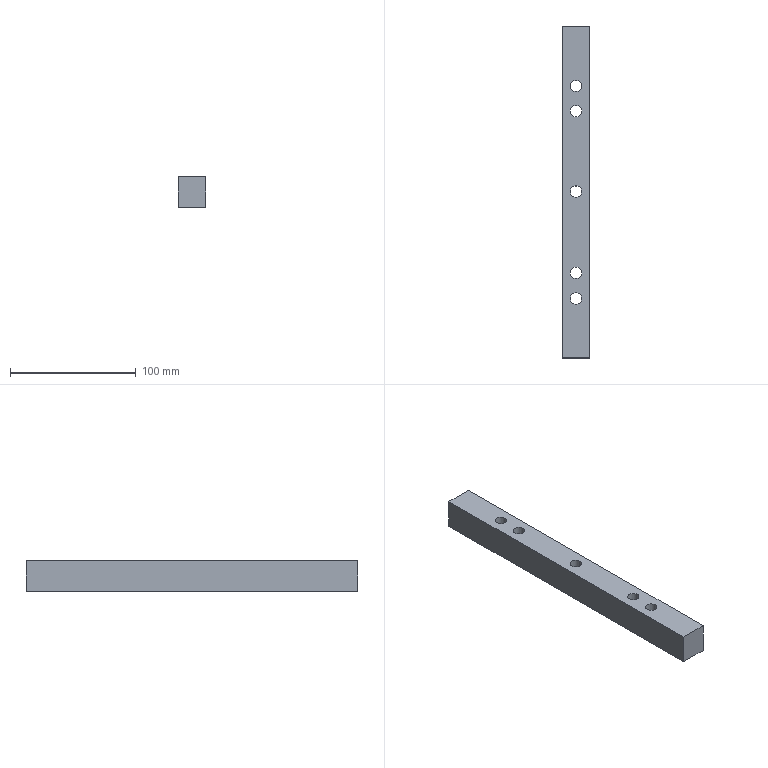Part | NX | features 1605158386 2 | 1 solid | 11 faces | box 22 x 264 x 24 mm | volume 131758 mm3 | plane 6 | cylinder 5 | commonest cylinder face diameters 9 x5
STEP:
#1=CARTESIAN_POINT('',(-281.,-132.15,-46.5));
#2=VERTEX_POINT('',#1);
#3=CARTESIAN_POINT('',(-281.,-132.15,-22.5));
#4=VERTEX_POINT('',#3);
#5=CARTESIAN_POINT('',(-281.,-132.15,-62.5));
#6=DIRECTION('',(0.,0.,1.));
#7=VECTOR('',#6,1000.);
#8=LINE('',#5,#7);
#9=EDGE_CURVE('',#2,#4,#8,.T.);
#10=ORIENTED_EDGE('',*,*,#9,.T.);
#11=CARTESIAN_POINT('',(-303.,-132.15,-22.5));
#12=VERTEX_POINT('',#11);
#13=CARTESIAN_POINT('',(-293.5,-132.15,-22.5));
#14=DIRECTION('',(-1.,0.,0.));
#15=VECTOR('',#14,1000.);
#16=LINE('',#13,#15);
#17=EDGE_CURVE('',#4,#12,#16,.T.);
#18=ORIENTED_EDGE('',*,*,#17,.T.);
#19=CARTESIAN_POINT('',(-303.,-132.15,-46.5));
#20=VERTEX_POINT('',#19);
#21=CARTESIAN_POINT('',(-303.,-132.15,-62.5));
#22=DIRECTION('',(0.,0.,1.));
#23=VECTOR('',#22,1000.);
#24=LINE('',#21,#23);
#25=EDGE_CURVE('',#20,#12,#24,.T.);
#26=ORIENTED_EDGE('',*,*,#25,.F.);
#27=CARTESIAN_POINT('',(-293.5,-132.15,-46.5));
#28=DIRECTION('',(1.,0.,0.));
#29=VECTOR('',#28,1000.);
#30=LINE('',#27,#29);
#31=EDGE_CURVE('',#20,#2,#30,.T.);
#32=ORIENTED_EDGE('',*,*,#31,.T.);
#33=EDGE_LOOP('',(#10,#18,#26,#32));
#34=FACE_BOUND('',#33,.T.);
#35=CARTESIAN_POINT('',(-293.5,-132.15,-62.5));
#36=DIRECTION('',(0.,-1.,0.));
#37=DIRECTION('',(0.,0.,-1.));
#38=AXIS2_PLACEMENT_3D('',#35,#36,#37);
#39=PLANE('',#38);
#40=ADVANCED_FACE('',(#34),#39,.T.);
#41=ORIENTED_EDGE('',*,*,#25,.T.);
#42=CARTESIAN_POINT('',(-303.,131.85,-22.5));
#43=VERTEX_POINT('',#42);
#44=CARTESIAN_POINT('',(-303.,108.85,-22.5));
#45=DIRECTION('',(0.,1.,0.));
#46=VECTOR('',#45,1000.);
#47=LINE('',#44,#46);
#48=EDGE_CURVE('',#12,#43,#47,.T.);
#49=ORIENTED_EDGE('',*,*,#48,.T.);
#50=CARTESIAN_POINT('',(-303.,131.85,-46.5));
#51=VERTEX_POINT('',#50);
#52=CARTESIAN_POINT('',(-303.,131.85,-62.5));
#53=DIRECTION('',(0.,0.,1.));
#54=VECTOR('',#53,1000.);
#55=LINE('',#52,#54);
#56=EDGE_CURVE('',#51,#43,#55,.T.);
#57=ORIENTED_EDGE('',*,*,#56,.F.);
#58=CARTESIAN_POINT('',(-303.,108.85,-46.5));
#59=DIRECTION('',(0.,-1.,0.));
#60=VECTOR('',#59,1000.);
#61=LINE('',#58,#60);
#62=EDGE_CURVE('',#51,#20,#61,.T.);
#63=ORIENTED_EDGE('',*,*,#62,.T.);
#64=EDGE_LOOP('',(#41,#49,#57,#63));
#65=FACE_BOUND('',#64,.T.);
#66=CARTESIAN_POINT('',(-303.,108.85,-62.5));
#67=DIRECTION('',(-1.,0.,0.));
#68=DIRECTION('',(0.,0.,1.));
#69=AXIS2_PLACEMENT_3D('',#66,#67,#68);
#70=PLANE('',#69);
#71=ADVANCED_FACE('',(#65),#70,.T.);
#72=ORIENTED_EDGE('',*,*,#56,.T.);
#73=CARTESIAN_POINT('',(-281.,131.85,-22.5));
#74=VERTEX_POINT('',#73);
#75=CARTESIAN_POINT('',(-293.5,131.85,-22.5));
#76=DIRECTION('',(1.,0.,0.));
#77=VECTOR('',#76,1000.);
#78=LINE('',#75,#77);
#79=EDGE_CURVE('',#43,#74,#78,.T.);
#80=ORIENTED_EDGE('',*,*,#79,.T.);
#81=CARTESIAN_POINT('',(-281.,131.85,-46.5));
#82=VERTEX_POINT('',#81);
#83=CARTESIAN_POINT('',(-281.,131.85,-62.5));
#84=DIRECTION('',(0.,0.,1.));
#85=VECTOR('',#84,1000.);
#86=LINE('',#83,#85);
#87=EDGE_CURVE('',#82,#74,#86,.T.);
#88=ORIENTED_EDGE('',*,*,#87,.F.);
#89=CARTESIAN_POINT('',(-293.5,131.85,-46.5));
#90=DIRECTION('',(-1.,0.,0.));
#91=VECTOR('',#90,1000.);
#92=LINE('',#89,#91);
#93=EDGE_CURVE('',#82,#51,#92,.T.);
#94=ORIENTED_EDGE('',*,*,#93,.T.);
#95=EDGE_LOOP('',(#72,#80,#88,#94));
#96=FACE_BOUND('',#95,.T.);
#97=CARTESIAN_POINT('',(-293.5,131.85,-62.5));
#98=DIRECTION('',(0.,1.,0.));
#99=DIRECTION('',(0.,0.,1.));
#100=AXIS2_PLACEMENT_3D('',#97,#98,#99);
#101=PLANE('',#100);
#102=ADVANCED_FACE('',(#96),#101,.T.);
#103=CARTESIAN_POINT('',(-296.5,0.15,-46.5));
#104=VERTEX_POINT('',#103);
#105=CARTESIAN_POINT('',(-292.,0.15,-46.5));
#106=DIRECTION('',(0.,0.,-1.));
#107=DIRECTION('',(-1.,0.,0.));
#108=AXIS2_PLACEMENT_3D('',#105,#106,#107);
#109=CIRCLE('',#108,4.5);
#110=EDGE_CURVE('',#104,#104,#109,.T.);
#111=ORIENTED_EDGE('',*,*,#110,.F.);
#112=EDGE_LOOP('',(#111));
#113=FACE_BOUND('',#112,.T.);
#114=CARTESIAN_POINT('',(-296.5,64.15,-46.5));
#115=VERTEX_POINT('',#114);
#116=CARTESIAN_POINT('',(-292.,64.15,-46.5));
#117=DIRECTION('',(0.,0.,-1.));
#118=DIRECTION('',(-1.,0.,0.));
#119=AXIS2_PLACEMENT_3D('',#116,#117,#118);
#120=CIRCLE('',#119,4.5);
#121=EDGE_CURVE('',#115,#115,#120,.T.);
#122=ORIENTED_EDGE('',*,*,#121,.F.);
#123=EDGE_LOOP('',(#122));
#124=FACE_BOUND('',#123,.T.);
#125=CARTESIAN_POINT('',(-296.5,84.15,-46.5));
#126=VERTEX_POINT('',#125);
#127=CARTESIAN_POINT('',(-292.,84.15,-46.5));
#128=DIRECTION('',(0.,0.,-1.));
#129=DIRECTION('',(-1.,0.,0.));
#130=AXIS2_PLACEMENT_3D('',#127,#128,#129);
#131=CIRCLE('',#130,4.5);
#132=EDGE_CURVE('',#126,#126,#131,.T.);
#133=ORIENTED_EDGE('',*,*,#132,.F.);
#134=EDGE_LOOP('',(#133));
#135=FACE_BOUND('',#134,.T.);
#136=CARTESIAN_POINT('',(-296.5,-84.85,-46.5));
#137=VERTEX_POINT('',#136);
#138=CARTESIAN_POINT('',(-292.,-84.85,-46.5));
#139=DIRECTION('',(0.,0.,-1.));
#140=DIRECTION('',(-1.,0.,0.));
#141=AXIS2_PLACEMENT_3D('',#138,#139,#140);
#142=CIRCLE('',#141,4.5);
#143=EDGE_CURVE('',#137,#137,#142,.T.);
#144=ORIENTED_EDGE('',*,*,#143,.F.);
#145=EDGE_LOOP('',(#144));
#146=FACE_BOUND('',#145,.T.);
#147=CARTESIAN_POINT('',(-296.5,-64.45,-46.5));
#148=VERTEX_POINT('',#147);
#149=CARTESIAN_POINT('',(-292.,-64.45,-46.5));
#150=DIRECTION('',(0.,0.,-1.));
#151=DIRECTION('',(-1.,0.,0.));
#152=AXIS2_PLACEMENT_3D('',#149,#150,#151);
#153=CIRCLE('',#152,4.5);
#154=EDGE_CURVE('',#148,#148,#153,.T.);
#155=ORIENTED_EDGE('',*,*,#154,.F.);
#156=EDGE_LOOP('',(#155));
#157=FACE_BOUND('',#156,.T.);
#158=CARTESIAN_POINT('',(-281.,108.85,-46.5));
#159=DIRECTION('',(0.,1.,0.));
#160=VECTOR('',#159,1000.);
#161=LINE('',#158,#160);
#162=EDGE_CURVE('',#2,#82,#161,.T.);
#163=ORIENTED_EDGE('',*,*,#162,.F.);
#164=ORIENTED_EDGE('',*,*,#31,.F.);
#165=ORIENTED_EDGE('',*,*,#62,.F.);
#166=ORIENTED_EDGE('',*,*,#93,.F.);
#167=EDGE_LOOP('',(#163,#164,#165,#166));
#168=FACE_BOUND('',#167,.T.);
#169=CARTESIAN_POINT('',(-293.5,108.85,-46.5));
#170=DIRECTION('',(0.,0.,-1.));
#171=DIRECTION('',(-1.,0.,0.));
#172=AXIS2_PLACEMENT_3D('',#169,#170,#171);
#173=PLANE('',#172);
#174=ADVANCED_FACE('',(#113,#124,#135,#146,#157,#168),#173,.T.);
#175=ORIENTED_EDGE('',*,*,#162,.T.);
#176=ORIENTED_EDGE('',*,*,#87,.T.);
#177=CARTESIAN_POINT('',(-281.,108.85,-22.5));
#178=DIRECTION('',(0.,-1.,0.));
#179=VECTOR('',#178,1000.);
#180=LINE('',#177,#179);
#181=EDGE_CURVE('',#74,#4,#180,.T.);
#182=ORIENTED_EDGE('',*,*,#181,.T.);
#183=ORIENTED_EDGE('',*,*,#9,.F.);
#184=EDGE_LOOP('',(#175,#176,#182,#183));
#185=FACE_BOUND('',#184,.T.);
#186=CARTESIAN_POINT('',(-281.,108.85,-62.5));
#187=DIRECTION('',(1.,0.,0.));
#188=DIRECTION('',(0.,0.,-1.));
#189=AXIS2_PLACEMENT_3D('',#186,#187,#188);
#190=PLANE('',#189);
#191=ADVANCED_FACE('',(#185),#190,.T.);
#192=CARTESIAN_POINT('',(-287.5,0.15,-22.5));
#193=VERTEX_POINT('',#192);
#194=CARTESIAN_POINT('',(-292.,0.15,-22.5));
#195=DIRECTION('',(0.,0.,1.));
#196=DIRECTION('',(1.,0.,0.));
#197=AXIS2_PLACEMENT_3D('',#194,#195,#196);
#198=CIRCLE('',#197,4.5);
#199=EDGE_CURVE('',#193,#193,#198,.T.);
#200=ORIENTED_EDGE('',*,*,#199,.F.);
#201=EDGE_LOOP('',(#200));
#202=FACE_BOUND('',#201,.T.);
#203=CARTESIAN_POINT('',(-287.5,64.15,-22.5));
#204=VERTEX_POINT('',#203);
#205=CARTESIAN_POINT('',(-292.,64.15,-22.5));
#206=DIRECTION('',(0.,0.,1.));
#207=DIRECTION('',(1.,0.,0.));
#208=AXIS2_PLACEMENT_3D('',#205,#206,#207);
#209=CIRCLE('',#208,4.5);
#210=EDGE_CURVE('',#204,#204,#209,.T.);
#211=ORIENTED_EDGE('',*,*,#210,.F.);
#212=EDGE_LOOP('',(#211));
#213=FACE_BOUND('',#212,.T.);
#214=CARTESIAN_POINT('',(-287.5,84.15,-22.5));
#215=VERTEX_POINT('',#214);
#216=CARTESIAN_POINT('',(-292.,84.15,-22.5));
#217=DIRECTION('',(0.,0.,1.));
#218=DIRECTION('',(1.,0.,0.));
#219=AXIS2_PLACEMENT_3D('',#216,#217,#218);
#220=CIRCLE('',#219,4.5);
#221=EDGE_CURVE('',#215,#215,#220,.T.);
#222=ORIENTED_EDGE('',*,*,#221,.F.);
#223=EDGE_LOOP('',(#222));
#224=FACE_BOUND('',#223,.T.);
#225=CARTESIAN_POINT('',(-287.5,-84.85,-22.5));
#226=VERTEX_POINT('',#225);
#227=CARTESIAN_POINT('',(-292.,-84.85,-22.5));
#228=DIRECTION('',(0.,0.,1.));
#229=DIRECTION('',(1.,0.,0.));
#230=AXIS2_PLACEMENT_3D('',#227,#228,#229);
#231=CIRCLE('',#230,4.5);
#232=EDGE_CURVE('',#226,#226,#231,.T.);
#233=ORIENTED_EDGE('',*,*,#232,.F.);
#234=EDGE_LOOP('',(#233));
#235=FACE_BOUND('',#234,.T.);
#236=CARTESIAN_POINT('',(-287.5,-64.45,-22.5));
#237=VERTEX_POINT('',#236);
#238=CARTESIAN_POINT('',(-292.,-64.45,-22.5));
#239=DIRECTION('',(0.,0.,1.));
#240=DIRECTION('',(1.,0.,0.));
#241=AXIS2_PLACEMENT_3D('',#238,#239,#240);
#242=CIRCLE('',#241,4.5);
#243=EDGE_CURVE('',#237,#237,#242,.T.);
#244=ORIENTED_EDGE('',*,*,#243,.F.);
#245=EDGE_LOOP('',(#244));
#246=FACE_BOUND('',#245,.T.);
#247=ORIENTED_EDGE('',*,*,#17,.F.);
#248=ORIENTED_EDGE('',*,*,#181,.F.);
#249=ORIENTED_EDGE('',*,*,#79,.F.);
#250=ORIENTED_EDGE('',*,*,#48,.F.);
#251=EDGE_LOOP('',(#247,#248,#249,#250));
#252=FACE_BOUND('',#251,.T.);
#253=CARTESIAN_POINT('',(-293.5,108.85,-22.5));
#254=DIRECTION('',(0.,0.,1.));
#255=DIRECTION('',(1.,0.,0.));
#256=AXIS2_PLACEMENT_3D('',#253,#254,#255);
#257=PLANE('',#256);
#258=ADVANCED_FACE('',(#202,#213,#224,#235,#246,#252),#257,.T.);
#259=ORIENTED_EDGE('',*,*,#154,.T.);
#260=EDGE_LOOP('',(#259));
#261=FACE_BOUND('',#260,.T.);
#262=ORIENTED_EDGE('',*,*,#243,.T.);
#263=EDGE_LOOP('',(#262));
#264=FACE_BOUND('',#263,.T.);
#265=CARTESIAN_POINT('',(-292.,-64.45,-22.4));
#266=DIRECTION('',(0.,0.,-1.));
#267=DIRECTION('',(1.,0.,0.));
#268=AXIS2_PLACEMENT_3D('',#265,#266,#267);
#269=CYLINDRICAL_SURFACE('',#268,4.5);
#270=ADVANCED_FACE('',(#261,#264),#269,.F.);
#271=ORIENTED_EDGE('',*,*,#143,.T.);
#272=EDGE_LOOP('',(#271));
#273=FACE_BOUND('',#272,.T.);
#274=ORIENTED_EDGE('',*,*,#232,.T.);
#275=EDGE_LOOP('',(#274));
#276=FACE_BOUND('',#275,.T.);
#277=CARTESIAN_POINT('',(-292.,-84.85,-22.4));
#278=DIRECTION('',(0.,0.,-1.));
#279=DIRECTION('',(1.,0.,0.));
#280=AXIS2_PLACEMENT_3D('',#277,#278,#279);
#281=CYLINDRICAL_SURFACE('',#280,4.5);
#282=ADVANCED_FACE('',(#273,#276),#281,.F.);
#283=ORIENTED_EDGE('',*,*,#132,.T.);
#284=EDGE_LOOP('',(#283));
#285=FACE_BOUND('',#284,.T.);
#286=ORIENTED_EDGE('',*,*,#221,.T.);
#287=EDGE_LOOP('',(#286));
#288=FACE_BOUND('',#287,.T.);
#289=CARTESIAN_POINT('',(-292.,84.15,-22.4));
#290=DIRECTION('',(0.,0.,-1.));
#291=DIRECTION('',(1.,0.,0.));
#292=AXIS2_PLACEMENT_3D('',#289,#290,#291);
#293=CYLINDRICAL_SURFACE('',#292,4.5);
#294=ADVANCED_FACE('',(#285,#288),#293,.F.);
#295=ORIENTED_EDGE('',*,*,#121,.T.);
#296=EDGE_LOOP('',(#295));
#297=FACE_BOUND('',#296,.T.);
#298=ORIENTED_EDGE('',*,*,#210,.T.);
#299=EDGE_LOOP('',(#298));
#300=FACE_BOUND('',#299,.T.);
#301=CARTESIAN_POINT('',(-292.,64.15,-22.4));
#302=DIRECTION('',(0.,0.,-1.));
#303=DIRECTION('',(1.,0.,0.));
#304=AXIS2_PLACEMENT_3D('',#301,#302,#303);
#305=CYLINDRICAL_SURFACE('',#304,4.5);
#306=ADVANCED_FACE('',(#297,#300),#305,.F.);
#307=ORIENTED_EDGE('',*,*,#110,.T.);
#308=EDGE_LOOP('',(#307));
#309=FACE_BOUND('',#308,.T.);
#310=ORIENTED_EDGE('',*,*,#199,.T.);
#311=EDGE_LOOP('',(#310));
#312=FACE_BOUND('',#311,.T.);
#313=CARTESIAN_POINT('',(-292.,0.15,-22.4));
#314=DIRECTION('',(0.,0.,-1.));
#315=DIRECTION('',(1.,0.,0.));
#316=AXIS2_PLACEMENT_3D('',#313,#314,#315);
#317=CYLINDRICAL_SURFACE('',#316,4.5);
#318=ADVANCED_FACE('',(#309,#312),#317,.F.);
#319=CLOSED_SHELL('',(#40,#71,#102,#174,#191,#258,#270,#282,#294,#306,#318));
#320=MANIFOLD_SOLID_BREP('',#319);
#321=(LENGTH_UNIT()NAMED_UNIT(*)SI_UNIT(.MILLI.,.METRE.));
#322=UNCERTAINTY_MEASURE_WITH_UNIT(LENGTH_MEASURE(0.00001),#321,'','');
#323=(NAMED_UNIT(*)PLANE_ANGLE_UNIT()SI_UNIT($,.RADIAN.));
#324=(NAMED_UNIT(*)SI_UNIT($,.STERADIAN.)SOLID_ANGLE_UNIT());
#325=(GEOMETRIC_REPRESENTATION_CONTEXT(3)GLOBAL_UNCERTAINTY_ASSIGNED_CONTEXT((#322))GLOBAL_UNIT_ASSIGNED_CONTEXT((#321,#323,#324))REPRESENTATION_CONTEXT('',''));
#326=ADVANCED_BREP_SHAPE_REPRESENTATION('',(#320),#325);